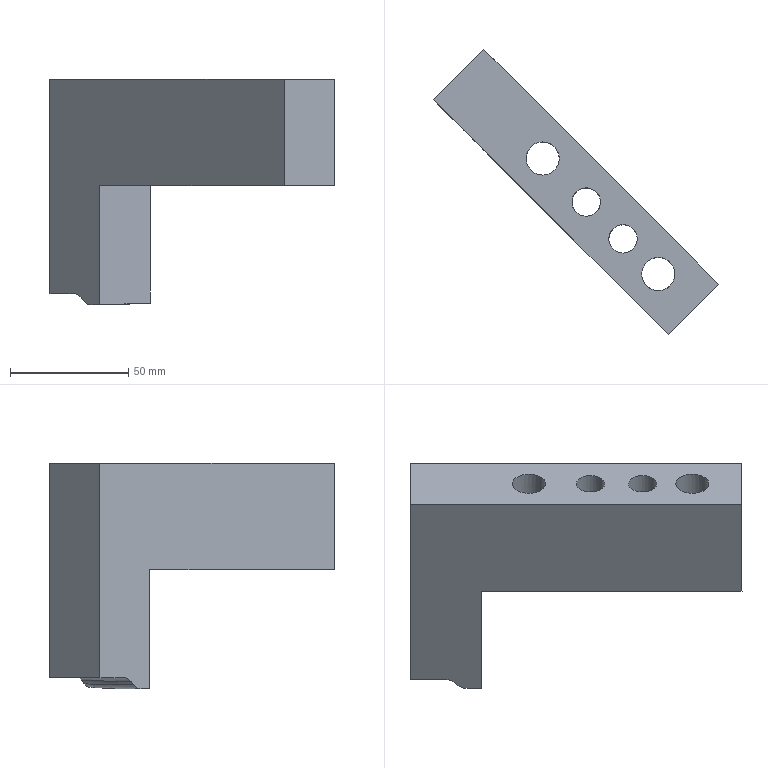Part | NX | features solid 2 | 1 solid | 21 faces | box 120.302 x 120.208 x 95.322 mm | volume 201033 mm3 | spline 8 | plane 7 | cylinder 6 | commonest cylinder face diameters 12 x2 14 x2 20 x2
STEP:
#1=CARTESIAN_POINT('',(-245.691,302.804,55.));
#2=VERTEX_POINT('',#1);
#3=CARTESIAN_POINT('',(-249.934,307.047,55.));
#4=DIRECTION('',(0.,0.,1.));
#5=DIRECTION('',(0.7071,-0.7071,0.));
#6=AXIS2_PLACEMENT_3D('',#3,#4,#5);
#7=CIRCLE('',#6,6.);
#8=EDGE_CURVE('',#2,#2,#7,.T.);
#9=ORIENTED_EDGE('',*,*,#8,.T.);
#10=EDGE_LOOP('',(#9));
#11=FACE_BOUND('',#10,.T.);
#12=CARTESIAN_POINT('',(-276.804,333.917,55.));
#13=VERTEX_POINT('',#12);
#14=CARTESIAN_POINT('',(-283.875,340.988,55.));
#15=DIRECTION('',(0.,0.,1.));
#16=DIRECTION('',(0.7071,-0.7071,0.));
#17=AXIS2_PLACEMENT_3D('',#14,#15,#16);
#18=CIRCLE('',#17,10.);
#19=EDGE_CURVE('',#13,#13,#18,.T.);
#20=ORIENTED_EDGE('',*,*,#19,.T.);
#21=EDGE_LOOP('',(#20));
#22=FACE_BOUND('',#21,.T.);
#23=CARTESIAN_POINT('',(-228.013,285.126,55.));
#24=VERTEX_POINT('',#23);
#25=CARTESIAN_POINT('',(-235.084,292.198,55.));
#26=DIRECTION('',(0.,0.,1.));
#27=DIRECTION('',(0.7071,-0.7071,0.));
#28=AXIS2_PLACEMENT_3D('',#25,#26,#27);
#29=CIRCLE('',#28,10.);
#30=EDGE_CURVE('',#24,#24,#29,.T.);
#31=ORIENTED_EDGE('',*,*,#30,.T.);
#32=EDGE_LOOP('',(#31));
#33=FACE_BOUND('',#32,.T.);
#34=CARTESIAN_POINT('',(-261.247,318.36,55.));
#35=VERTEX_POINT('',#34);
#36=CARTESIAN_POINT('',(-265.49,322.603,55.));
#37=DIRECTION('',(0.,0.,1.));
#38=DIRECTION('',(0.7071,-0.7071,0.));
#39=AXIS2_PLACEMENT_3D('',#36,#37,#38);
#40=CIRCLE('',#39,6.);
#41=EDGE_CURVE('',#35,#35,#40,.T.);
#42=ORIENTED_EDGE('',*,*,#41,.T.);
#43=EDGE_LOOP('',(#42));
#44=FACE_BOUND('',#43,.T.);
#45=CARTESIAN_POINT('',(-230.875,266.775,55.));
#46=VERTEX_POINT('',#45);
#47=CARTESIAN_POINT('',(-308.751,344.651,55.));
#48=VERTEX_POINT('',#47);
#49=CARTESIAN_POINT('',(-244.984,280.884,55.));
#50=DIRECTION('',(0.7071,-0.7071,0.));
#51=VECTOR('',#50,1000.);
#52=LINE('',#49,#51);
#53=EDGE_CURVE('',#46,#48,#52,.F.);
#54=ORIENTED_EDGE('',*,*,#53,.T.);
#55=CARTESIAN_POINT('',(-287.444,365.77,55.));
#56=VERTEX_POINT('',#55);
#57=CARTESIAN_POINT('',(-308.751,344.651,55.));
#58=CARTESIAN_POINT('',(-301.65,351.692,55.));
#59=CARTESIAN_POINT('',(-294.548,358.732,55.));
#60=CARTESIAN_POINT('',(-287.444,365.77,55.));
#61=B_SPLINE_CURVE_WITH_KNOTS('',3,(#57,#58,#59,#60),.UNSPECIFIED.,.F.,.F.,(4,4),(0.,0.03),.UNSPECIFIED.);
#62=EDGE_CURVE('',#48,#56,#61,.T.);
#63=ORIENTED_EDGE('',*,*,#62,.T.);
#64=CARTESIAN_POINT('',(-209.662,287.989,55.));
#65=VERTEX_POINT('',#64);
#66=CARTESIAN_POINT('',(-223.771,302.097,55.));
#67=DIRECTION('',(0.7071,-0.7071,0.));
#68=VECTOR('',#67,1000.);
#69=LINE('',#66,#68);
#70=EDGE_CURVE('',#65,#56,#69,.F.);
#71=ORIENTED_EDGE('',*,*,#70,.F.);
#72=CARTESIAN_POINT('',(-259.16,238.491,55.));
#73=DIRECTION('',(-0.7071,-0.7071,0.));
#74=VECTOR('',#73,1000.);
#75=LINE('',#72,#74);
#76=EDGE_CURVE('',#46,#65,#75,.F.);
#77=ORIENTED_EDGE('',*,*,#76,.F.);
#78=EDGE_LOOP('',(#54,#63,#71,#77));
#79=FACE_BOUND('',#78,.T.);
#80=CARTESIAN_POINT('',(-244.984,280.884,55.));
#81=DIRECTION('',(0.,0.,1.));
#82=DIRECTION('',(0.7071,0.7071,0.));
#83=AXIS2_PLACEMENT_3D('',#80,#81,#82);
#84=PLANE('',#83);
#85=ADVANCED_FACE('',(#11,#22,#33,#44,#79),#84,.F.);
#86=CARTESIAN_POINT('',(-329.964,365.864,100.));
#87=VERTEX_POINT('',#86);
#88=CARTESIAN_POINT('',(-308.657,386.983,100.));
#89=VERTEX_POINT('',#88);
#90=CARTESIAN_POINT('',(-329.964,365.864,100.));
#91=CARTESIAN_POINT('',(-322.863,372.905,100.));
#92=CARTESIAN_POINT('',(-315.761,379.945,100.));
#93=CARTESIAN_POINT('',(-308.657,386.983,100.));
#94=B_SPLINE_CURVE_WITH_KNOTS('',3,(#90,#91,#92,#93),.UNSPECIFIED.,.F.,.F.,(4,4),(0.04583,0.07583),.UNSPECIFIED.);
#95=EDGE_CURVE('',#87,#89,#94,.T.);
#96=ORIENTED_EDGE('',*,*,#95,.F.);
#97=CARTESIAN_POINT('',(-230.875,266.775,100.));
#98=VERTEX_POINT('',#97);
#99=CARTESIAN_POINT('',(-322.766,358.666,100.));
#100=DIRECTION('',(-0.7071,0.7071,0.));
#101=VECTOR('',#100,1000.);
#102=LINE('',#99,#101);
#103=EDGE_CURVE('',#98,#87,#102,.T.);
#104=ORIENTED_EDGE('',*,*,#103,.F.);
#105=CARTESIAN_POINT('',(-209.662,287.989,100.));
#106=VERTEX_POINT('',#105);
#107=CARTESIAN_POINT('',(-177.842,319.808,100.));
#108=DIRECTION('',(0.7071,0.7071,0.));
#109=VECTOR('',#108,1000.);
#110=LINE('',#107,#109);
#111=EDGE_CURVE('',#98,#106,#110,.T.);
#112=ORIENTED_EDGE('',*,*,#111,.T.);
#113=CARTESIAN_POINT('',(-301.552,379.879,100.));
#114=DIRECTION('',(-0.7071,0.7071,0.));
#115=VECTOR('',#114,1000.);
#116=LINE('',#113,#115);
#117=EDGE_CURVE('',#106,#89,#116,.T.);
#118=ORIENTED_EDGE('',*,*,#117,.T.);
#119=EDGE_LOOP('',(#96,#104,#112,#118));
#120=FACE_BOUND('',#119,.T.);
#121=CARTESIAN_POINT('',(-249.934,301.047,100.));
#122=VERTEX_POINT('',#121);
#123=CARTESIAN_POINT('',(-249.934,307.047,100.));
#124=DIRECTION('',(0.,0.,1.));
#125=DIRECTION('',(0.,-1.,0.));
#126=AXIS2_PLACEMENT_3D('',#123,#124,#125);
#127=CIRCLE('',#126,6.);
#128=EDGE_CURVE('',#122,#122,#127,.T.);
#129=ORIENTED_EDGE('',*,*,#128,.F.);
#130=EDGE_LOOP('',(#129));
#131=FACE_BOUND('',#130,.T.);
#132=CARTESIAN_POINT('',(-235.084,285.198,100.));
#133=VERTEX_POINT('',#132);
#134=CARTESIAN_POINT('',(-235.084,292.198,100.));
#135=DIRECTION('',(0.,0.,1.));
#136=DIRECTION('',(0.,-1.,0.));
#137=AXIS2_PLACEMENT_3D('',#134,#135,#136);
#138=CIRCLE('',#137,7.);
#139=EDGE_CURVE('',#133,#133,#138,.T.);
#140=ORIENTED_EDGE('',*,*,#139,.F.);
#141=EDGE_LOOP('',(#140));
#142=FACE_BOUND('',#141,.T.);
#143=CARTESIAN_POINT('',(-283.875,333.988,100.));
#144=VERTEX_POINT('',#143);
#145=CARTESIAN_POINT('',(-283.875,340.988,100.));
#146=DIRECTION('',(0.,0.,1.));
#147=DIRECTION('',(0.,-1.,0.));
#148=AXIS2_PLACEMENT_3D('',#145,#146,#147);
#149=CIRCLE('',#148,7.);
#150=EDGE_CURVE('',#144,#144,#149,.T.);
#151=ORIENTED_EDGE('',*,*,#150,.F.);
#152=EDGE_LOOP('',(#151));
#153=FACE_BOUND('',#152,.T.);
#154=CARTESIAN_POINT('',(-265.49,316.603,100.));
#155=VERTEX_POINT('',#154);
#156=CARTESIAN_POINT('',(-265.49,322.603,100.));
#157=DIRECTION('',(0.,0.,1.));
#158=DIRECTION('',(0.,-1.,0.));
#159=AXIS2_PLACEMENT_3D('',#156,#157,#158);
#160=CIRCLE('',#159,6.);
#161=EDGE_CURVE('',#155,#155,#160,.T.);
#162=ORIENTED_EDGE('',*,*,#161,.F.);
#163=EDGE_LOOP('',(#162));
#164=FACE_BOUND('',#163,.T.);
#165=CARTESIAN_POINT('',(-269.733,411.699,100.));
#166=DIRECTION('',(0.,0.,1.));
#167=DIRECTION('',(0.7071,-0.7071,0.));
#168=AXIS2_PLACEMENT_3D('',#165,#166,#167);
#169=PLANE('',#168);
#170=ADVANCED_FACE('',(#120,#131,#142,#153,#164),#169,.T.);
#171=CARTESIAN_POINT('',(-230.875,266.775,75.));
#172=DIRECTION('',(0.,0.,1.));
#173=VECTOR('',#172,1000.);
#174=LINE('',#171,#173);
#175=EDGE_CURVE('',#46,#98,#174,.T.);
#176=ORIENTED_EDGE('',*,*,#175,.F.);
#177=ORIENTED_EDGE('',*,*,#76,.T.);
#178=CARTESIAN_POINT('',(-209.662,287.989,75.));
#179=DIRECTION('',(0.,0.,1.));
#180=VECTOR('',#179,1000.);
#181=LINE('',#178,#180);
#182=EDGE_CURVE('',#65,#106,#181,.T.);
#183=ORIENTED_EDGE('',*,*,#182,.T.);
#184=ORIENTED_EDGE('',*,*,#111,.F.);
#185=EDGE_LOOP('',(#176,#177,#183,#184));
#186=FACE_BOUND('',#185,.T.);
#187=CARTESIAN_POINT('',(-259.16,238.491,75.));
#188=DIRECTION('',(0.7071,-0.7071,0.));
#189=DIRECTION('',(0.,0.,-1.));
#190=AXIS2_PLACEMENT_3D('',#187,#188,#189);
#191=PLANE('',#190);
#192=ADVANCED_FACE('',(#186),#191,.T.);
#193=CARTESIAN_POINT('',(-312.943,348.843,4.801));
#194=VERTEX_POINT('',#193);
#195=CARTESIAN_POINT('',(-315.708,351.608,6.413));
#196=VERTEX_POINT('',#195);
#197=CARTESIAN_POINT('',(-312.942,348.842,4.801));
#198=CARTESIAN_POINT('',(-313.969,349.869,4.845));
#199=CARTESIAN_POINT('',(-314.962,350.862,5.425));
#200=CARTESIAN_POINT('',(-315.711,351.611,6.417));
#201=B_SPLINE_CURVE_WITH_KNOTS('',3,(#197,#198,#199,#200),.UNSPECIFIED.,.F.,.F.,(4,4),(0.,0.004334),.UNSPECIFIED.);
#202=EDGE_CURVE('',#194,#196,#201,.T.);
#203=ORIENTED_EDGE('',*,*,#202,.F.);
#204=CARTESIAN_POINT('',(-308.751,344.651,4.678));
#205=VERTEX_POINT('',#204);
#206=CARTESIAN_POINT('',(-312.944,348.844,4.801));
#207=CARTESIAN_POINT('',(-311.546,347.446,4.74));
#208=CARTESIAN_POINT('',(-310.149,346.049,4.7));
#209=CARTESIAN_POINT('',(-308.751,344.651,4.678));
#210=B_SPLINE_CURVE_WITH_KNOTS('',3,(#206,#207,#208,#209),.UNSPECIFIED.,.F.,.F.,(4,4),(0.02411,0.03004),.UNSPECIFIED.);
#211=EDGE_CURVE('',#194,#205,#210,.T.);
#212=ORIENTED_EDGE('',*,*,#211,.T.);
#213=CARTESIAN_POINT('',(-308.751,344.651,54.885));
#214=DIRECTION('',(0.,0.,-1.));
#215=VECTOR('',#214,1000.);
#216=LINE('',#213,#215);
#217=EDGE_CURVE('',#48,#205,#216,.T.);
#218=ORIENTED_EDGE('',*,*,#217,.F.);
#219=ORIENTED_EDGE('',*,*,#53,.F.);
#220=ORIENTED_EDGE('',*,*,#175,.T.);
#221=ORIENTED_EDGE('',*,*,#103,.T.);
#222=CARTESIAN_POINT('',(-329.964,365.864,9.341));
#223=VERTEX_POINT('',#222);
#224=CARTESIAN_POINT('',(-329.964,365.864,70.));
#225=DIRECTION('',(0.,0.,-1.));
#226=VECTOR('',#225,1000.);
#227=LINE('',#224,#226);
#228=EDGE_CURVE('',#87,#223,#227,.T.);
#229=ORIENTED_EDGE('',*,*,#228,.T.);
#230=CARTESIAN_POINT('',(-328.671,364.571,9.579));
#231=VERTEX_POINT('',#230);
#232=CARTESIAN_POINT('',(-329.964,365.864,9.341));
#233=CARTESIAN_POINT('',(-329.542,365.442,9.515));
#234=CARTESIAN_POINT('',(-329.111,365.011,9.594));
#235=CARTESIAN_POINT('',(-328.672,364.572,9.579));
#236=B_SPLINE_CURVE_WITH_KNOTS('',3,(#232,#233,#234,#235),.UNSPECIFIED.,.F.,.F.,(4,4),(0.,0.001844),.UNSPECIFIED.);
#237=EDGE_CURVE('',#223,#231,#236,.T.);
#238=ORIENTED_EDGE('',*,*,#237,.T.);
#239=CARTESIAN_POINT('',(-319.575,355.475,9.376));
#240=VERTEX_POINT('',#239);
#241=CARTESIAN_POINT('',(-328.669,364.569,9.579));
#242=CARTESIAN_POINT('',(-325.638,361.538,9.472));
#243=CARTESIAN_POINT('',(-322.607,358.507,9.405));
#244=CARTESIAN_POINT('',(-319.575,355.475,9.376));
#245=B_SPLINE_CURVE_WITH_KNOTS('',3,(#241,#242,#243,#244),.UNSPECIFIED.,.F.,.F.,(4,4),(0.001832,0.01469),.UNSPECIFIED.);
#246=EDGE_CURVE('',#231,#240,#245,.T.);
#247=ORIENTED_EDGE('',*,*,#246,.T.);
#248=CARTESIAN_POINT('',(-316.651,352.551,7.683));
#249=VERTEX_POINT('',#248);
#250=CARTESIAN_POINT('',(-319.576,355.476,9.376));
#251=CARTESIAN_POINT('',(-318.489,354.389,9.366));
#252=CARTESIAN_POINT('',(-317.43,353.33,8.753));
#253=CARTESIAN_POINT('',(-316.65,352.55,7.682));
#254=B_SPLINE_CURVE_WITH_KNOTS('',3,(#250,#251,#252,#253),.UNSPECIFIED.,.F.,.F.,(4,4),(0.,0.004586),.UNSPECIFIED.);
#255=EDGE_CURVE('',#240,#249,#254,.T.);
#256=ORIENTED_EDGE('',*,*,#255,.T.);
#257=CARTESIAN_POINT('',(-316.651,352.551,7.683));
#258=CARTESIAN_POINT('',(-316.339,352.239,7.255));
#259=CARTESIAN_POINT('',(-316.024,351.924,6.831));
#260=CARTESIAN_POINT('',(-315.707,351.607,6.411));
#261=B_SPLINE_CURVE_WITH_KNOTS('',3,(#257,#258,#259,#260),.UNSPECIFIED.,.F.,.F.,(4,4),(0.01484,0.01668),.UNSPECIFIED.);
#262=EDGE_CURVE('',#249,#196,#261,.T.);
#263=ORIENTED_EDGE('',*,*,#262,.T.);
#264=EDGE_LOOP('',(#203,#212,#218,#219,#220,#221,#229,#238,#247,#256,#263));
#265=FACE_BOUND('',#264,.T.);
#266=CARTESIAN_POINT('',(-266.197,302.097,75.));
#267=DIRECTION('',(0.7071,0.7071,0.));
#268=DIRECTION('',(0.,0.,1.));
#269=AXIS2_PLACEMENT_3D('',#266,#267,#268);
#270=PLANE('',#269);
#271=ADVANCED_FACE('',(#265),#270,.F.);
#272=CARTESIAN_POINT('',(-291.158,369.484,5.289));
#273=VERTEX_POINT('',#272);
#274=CARTESIAN_POINT('',(-287.444,365.77,5.473));
#275=VERTEX_POINT('',#274);
#276=CARTESIAN_POINT('',(-291.157,369.484,5.289));
#277=CARTESIAN_POINT('',(-289.919,368.246,5.342));
#278=CARTESIAN_POINT('',(-288.681,367.008,5.403));
#279=CARTESIAN_POINT('',(-287.444,365.77,5.473));
#280=B_SPLINE_CURVE_WITH_KNOTS('',3,(#276,#277,#278,#279),.UNSPECIFIED.,.F.,.F.,(4,4),(0.01502,0.02027),.UNSPECIFIED.);
#281=EDGE_CURVE('',#273,#275,#280,.T.);
#282=ORIENTED_EDGE('',*,*,#281,.F.);
#283=CARTESIAN_POINT('',(-294.149,372.475,6.862));
#284=VERTEX_POINT('',#283);
#285=CARTESIAN_POINT('',(-291.158,369.484,5.289));
#286=CARTESIAN_POINT('',(-292.256,370.582,5.242));
#287=CARTESIAN_POINT('',(-293.342,371.668,5.814));
#288=CARTESIAN_POINT('',(-294.151,372.477,6.865));
#289=B_SPLINE_CURVE_WITH_KNOTS('',3,(#285,#286,#287,#288),.UNSPECIFIED.,.F.,.F.,(4,4),(0.,0.004637),.UNSPECIFIED.);
#290=EDGE_CURVE('',#273,#284,#289,.T.);
#291=ORIENTED_EDGE('',*,*,#290,.T.);
#292=CARTESIAN_POINT('',(-295.242,373.569,8.306));
#293=VERTEX_POINT('',#292);
#294=CARTESIAN_POINT('',(-295.242,373.569,8.306));
#295=CARTESIAN_POINT('',(-294.88,373.206,7.819));
#296=CARTESIAN_POINT('',(-294.515,372.841,7.337));
#297=CARTESIAN_POINT('',(-294.146,372.473,6.858));
#298=B_SPLINE_CURVE_WITH_KNOTS('',3,(#294,#295,#296,#297),.UNSPECIFIED.,.F.,.F.,(4,4),(0.008363,0.01048),.UNSPECIFIED.);
#299=EDGE_CURVE('',#293,#284,#298,.T.);
#300=ORIENTED_EDGE('',*,*,#299,.F.);
#301=CARTESIAN_POINT('',(-298.297,376.624,9.952));
#302=VERTEX_POINT('',#301);
#303=CARTESIAN_POINT('',(-298.297,376.624,9.952));
#304=CARTESIAN_POINT('',(-297.172,375.498,10.002));
#305=CARTESIAN_POINT('',(-296.058,374.385,9.403));
#306=CARTESIAN_POINT('',(-295.242,373.568,8.306));
#307=B_SPLINE_CURVE_WITH_KNOTS('',3,(#303,#304,#305,#306),.UNSPECIFIED.,.F.,.F.,(4,4),(0.,0.004753),.UNSPECIFIED.);
#308=EDGE_CURVE('',#302,#293,#307,.T.);
#309=ORIENTED_EDGE('',*,*,#308,.F.);
#310=CARTESIAN_POINT('',(-307.448,385.775,9.639));
#311=VERTEX_POINT('',#310);
#312=CARTESIAN_POINT('',(-307.448,385.775,9.639));
#313=CARTESIAN_POINT('',(-304.397,382.724,9.71));
#314=CARTESIAN_POINT('',(-301.347,379.674,9.815));
#315=CARTESIAN_POINT('',(-298.298,376.624,9.952));
#316=B_SPLINE_CURVE_WITH_KNOTS('',3,(#312,#313,#314,#315),.UNSPECIFIED.,.F.,.F.,(4,4),(0.001709,0.01465),.UNSPECIFIED.);
#317=EDGE_CURVE('',#311,#302,#316,.T.);
#318=ORIENTED_EDGE('',*,*,#317,.F.);
#319=CARTESIAN_POINT('',(-308.657,386.983,9.361));
#320=VERTEX_POINT('',#319);
#321=CARTESIAN_POINT('',(-308.657,386.983,9.361));
#322=CARTESIAN_POINT('',(-308.264,386.59,9.537));
#323=CARTESIAN_POINT('',(-307.861,386.187,9.63));
#324=CARTESIAN_POINT('',(-307.448,385.775,9.639));
#325=B_SPLINE_CURVE_WITH_KNOTS('',3,(#321,#322,#323,#324),.UNSPECIFIED.,.F.,.F.,(4,4),(0.,0.001732),.UNSPECIFIED.);
#326=EDGE_CURVE('',#320,#311,#325,.T.);
#327=ORIENTED_EDGE('',*,*,#326,.F.);
#328=CARTESIAN_POINT('',(-308.657,386.983,500.));
#329=DIRECTION('',(0.,0.,-1.));
#330=VECTOR('',#329,1000.);
#331=LINE('',#328,#330);
#332=EDGE_CURVE('',#89,#320,#331,.T.);
#333=ORIENTED_EDGE('',*,*,#332,.F.);
#334=ORIENTED_EDGE('',*,*,#117,.F.);
#335=ORIENTED_EDGE('',*,*,#182,.F.);
#336=ORIENTED_EDGE('',*,*,#70,.T.);
#337=CARTESIAN_POINT('',(-287.444,365.77,55.532));
#338=DIRECTION('',(0.,0.,-1.));
#339=VECTOR('',#338,1000.);
#340=LINE('',#337,#339);
#341=EDGE_CURVE('',#56,#275,#340,.T.);
#342=ORIENTED_EDGE('',*,*,#341,.T.);
#343=EDGE_LOOP('',(#282,#291,#300,#309,#318,#327,#333,#334,#335,#336,#342));
#344=FACE_BOUND('',#343,.T.);
#345=CARTESIAN_POINT('',(-244.984,323.31,-200.));
#346=DIRECTION('',(0.7071,0.7071,0.));
#347=DIRECTION('',(0.,0.,1.));
#348=AXIS2_PLACEMENT_3D('',#345,#346,#347);
#349=PLANE('',#348);
#350=ADVANCED_FACE('',(#344),#349,.T.);
#351=CARTESIAN_POINT('',(-228.013,285.126,75.));
#352=VERTEX_POINT('',#351);
#353=CARTESIAN_POINT('',(-235.084,292.198,75.));
#354=DIRECTION('',(0.,0.,1.));
#355=DIRECTION('',(0.7071,-0.7071,0.));
#356=AXIS2_PLACEMENT_3D('',#353,#354,#355);
#357=CIRCLE('',#356,10.);
#358=EDGE_CURVE('',#352,#352,#357,.F.);
#359=ORIENTED_EDGE('',*,*,#358,.F.);
#360=EDGE_LOOP('',(#359));
#361=FACE_BOUND('',#360,.T.);
#362=ORIENTED_EDGE('',*,*,#30,.F.);
#363=EDGE_LOOP('',(#362));
#364=FACE_BOUND('',#363,.T.);
#365=CARTESIAN_POINT('',(-235.084,292.198,72.));
#366=DIRECTION('',(0.,0.,-1.));
#367=DIRECTION('',(0.7071,-0.7071,0.));
#368=AXIS2_PLACEMENT_3D('',#365,#366,#367);
#369=CYLINDRICAL_SURFACE('',#368,10.);
#370=ADVANCED_FACE('',(#361,#364),#369,.F.);
#371=CARTESIAN_POINT('',(-276.804,333.917,75.));
#372=VERTEX_POINT('',#371);
#373=CARTESIAN_POINT('',(-283.875,340.988,75.));
#374=DIRECTION('',(0.,0.,-1.));
#375=DIRECTION('',(0.7071,-0.7071,0.));
#376=AXIS2_PLACEMENT_3D('',#373,#374,#375);
#377=CIRCLE('',#376,10.);
#378=EDGE_CURVE('',#372,#372,#377,.T.);
#379=ORIENTED_EDGE('',*,*,#378,.F.);
#380=EDGE_LOOP('',(#379));
#381=FACE_BOUND('',#380,.T.);
#382=ORIENTED_EDGE('',*,*,#19,.F.);
#383=EDGE_LOOP('',(#382));
#384=FACE_BOUND('',#383,.T.);
#385=CARTESIAN_POINT('',(-283.875,340.988,75.));
#386=DIRECTION('',(0.,0.,-1.));
#387=DIRECTION('',(0.7071,-0.7071,0.));
#388=AXIS2_PLACEMENT_3D('',#385,#386,#387);
#389=CYLINDRICAL_SURFACE('',#388,10.);
#390=ADVANCED_FACE('',(#381,#384),#389,.F.);
#391=ORIENTED_EDGE('',*,*,#332,.T.);
#392=CARTESIAN_POINT('',(-308.657,386.983,9.361));
#393=CARTESIAN_POINT('',(-315.76,379.946,9.178));
#394=CARTESIAN_POINT('',(-322.864,372.905,9.162));
#395=CARTESIAN_POINT('',(-329.964,365.864,9.341));
#396=B_SPLINE_CURVE_WITH_KNOTS('',3,(#392,#393,#394,#395),.UNSPECIFIED.,.F.,.F.,(4,4),(0.,0.03),.UNSPECIFIED.);
#397=EDGE_CURVE('',#320,#223,#396,.T.);
#398=ORIENTED_EDGE('',*,*,#397,.T.);
#399=ORIENTED_EDGE('',*,*,#228,.F.);
#400=ORIENTED_EDGE('',*,*,#95,.T.);
#401=EDGE_LOOP('',(#391,#398,#399,#400));
#402=FACE_BOUND('',#401,.T.);
#403=CARTESIAN_POINT('',(-308.657,386.983,100.));
#404=CARTESIAN_POINT('',(-308.657,386.983,8.651));
#405=CARTESIAN_POINT('',(-315.763,379.943,100.));
#406=CARTESIAN_POINT('',(-315.763,379.943,8.651));
#407=CARTESIAN_POINT('',(-322.865,372.903,100.));
#408=CARTESIAN_POINT('',(-322.865,372.903,8.651));
#409=CARTESIAN_POINT('',(-329.964,365.864,100.));
#410=CARTESIAN_POINT('',(-329.964,365.864,8.651));
#411=B_SPLINE_SURFACE_WITH_KNOTS('',3,1,((#403,#404),(#405,#406),(#407,#408),(#409,#410)),.SURF_OF_LINEAR_EXTRUSION.,.F.,.F.,.F.,(4,4),(2,2),(0.9474,0.9616),(0.,1.),.PIECEWISE_BEZIER_KNOTS.);
#412=ADVANCED_FACE('',(#402),#411,.F.);
#413=CARTESIAN_POINT('',(-230.135,287.248,75.));
#414=VERTEX_POINT('',#413);
#415=CARTESIAN_POINT('',(-235.084,292.198,75.));
#416=DIRECTION('',(0.,0.,1.));
#417=DIRECTION('',(0.7071,-0.7071,0.));
#418=AXIS2_PLACEMENT_3D('',#415,#416,#417);
#419=CIRCLE('',#418,7.);
#420=EDGE_CURVE('',#414,#414,#419,.T.);
#421=ORIENTED_EDGE('',*,*,#420,.T.);
#422=EDGE_LOOP('',(#421));
#423=FACE_BOUND('',#422,.T.);
#424=ORIENTED_EDGE('',*,*,#358,.T.);
#425=EDGE_LOOP('',(#424));
#426=FACE_BOUND('',#425,.T.);
#427=CARTESIAN_POINT('',(-235.084,292.198,75.));
#428=DIRECTION('',(0.,0.,1.));
#429=DIRECTION('',(-0.7071,0.7071,0.));
#430=AXIS2_PLACEMENT_3D('',#427,#428,#429);
#431=PLANE('',#430);
#432=ADVANCED_FACE('',(#423,#426),#431,.F.);
#433=ORIENTED_EDGE('',*,*,#139,.T.);
#434=EDGE_LOOP('',(#433));
#435=FACE_BOUND('',#434,.T.);
#436=ORIENTED_EDGE('',*,*,#420,.F.);
#437=EDGE_LOOP('',(#436));
#438=FACE_BOUND('',#437,.T.);
#439=CARTESIAN_POINT('',(-235.084,292.198,72.));
#440=DIRECTION('',(0.,0.,1.));
#441=DIRECTION('',(-0.7071,0.7071,0.));
#442=AXIS2_PLACEMENT_3D('',#439,#440,#441);
#443=CYLINDRICAL_SURFACE('',#442,7.);
#444=ADVANCED_FACE('',(#435,#438),#443,.F.);
#445=CARTESIAN_POINT('',(-278.925,336.038,75.));
#446=VERTEX_POINT('',#445);
#447=CARTESIAN_POINT('',(-283.875,340.988,75.));
#448=DIRECTION('',(0.,0.,1.));
#449=DIRECTION('',(0.7071,-0.7071,0.));
#450=AXIS2_PLACEMENT_3D('',#447,#448,#449);
#451=CIRCLE('',#450,7.);
#452=EDGE_CURVE('',#446,#446,#451,.T.);
#453=ORIENTED_EDGE('',*,*,#452,.T.);
#454=EDGE_LOOP('',(#453));
#455=FACE_BOUND('',#454,.T.);
#456=ORIENTED_EDGE('',*,*,#378,.T.);
#457=EDGE_LOOP('',(#456));
#458=FACE_BOUND('',#457,.T.);
#459=CARTESIAN_POINT('',(-283.875,340.988,75.));
#460=DIRECTION('',(0.,0.,1.));
#461=DIRECTION('',(-0.7071,0.7071,0.));
#462=AXIS2_PLACEMENT_3D('',#459,#460,#461);
#463=PLANE('',#462);
#464=ADVANCED_FACE('',(#455,#458),#463,.F.);
#465=ORIENTED_EDGE('',*,*,#150,.T.);
#466=EDGE_LOOP('',(#465));
#467=FACE_BOUND('',#466,.T.);
#468=ORIENTED_EDGE('',*,*,#452,.F.);
#469=EDGE_LOOP('',(#468));
#470=FACE_BOUND('',#469,.T.);
#471=CARTESIAN_POINT('',(-283.875,340.988,75.));
#472=DIRECTION('',(0.,0.,1.));
#473=DIRECTION('',(-0.7071,0.7071,0.));
#474=AXIS2_PLACEMENT_3D('',#471,#472,#473);
#475=CYLINDRICAL_SURFACE('',#474,7.);
#476=ADVANCED_FACE('',(#467,#470),#475,.F.);
#477=ORIENTED_EDGE('',*,*,#161,.T.);
#478=EDGE_LOOP('',(#477));
#479=FACE_BOUND('',#478,.T.);
#480=ORIENTED_EDGE('',*,*,#41,.F.);
#481=EDGE_LOOP('',(#480));
#482=FACE_BOUND('',#481,.T.);
#483=CARTESIAN_POINT('',(-265.49,322.603,105.));
#484=DIRECTION('',(0.,0.,-1.));
#485=DIRECTION('',(-0.7071,0.7071,0.));
#486=AXIS2_PLACEMENT_3D('',#483,#484,#485);
#487=CYLINDRICAL_SURFACE('',#486,6.);
#488=ADVANCED_FACE('',(#479,#482),#487,.F.);
#489=ORIENTED_EDGE('',*,*,#128,.T.);
#490=EDGE_LOOP('',(#489));
#491=FACE_BOUND('',#490,.T.);
#492=ORIENTED_EDGE('',*,*,#8,.F.);
#493=EDGE_LOOP('',(#492));
#494=FACE_BOUND('',#493,.T.);
#495=CARTESIAN_POINT('',(-249.934,307.047,105.));
#496=DIRECTION('',(0.,0.,-1.));
#497=DIRECTION('',(-0.7071,0.7071,0.));
#498=AXIS2_PLACEMENT_3D('',#495,#496,#497);
#499=CYLINDRICAL_SURFACE('',#498,6.);
#500=ADVANCED_FACE('',(#491,#494),#499,.F.);
#501=ORIENTED_EDGE('',*,*,#217,.T.);
#502=CARTESIAN_POINT('',(-308.751,344.651,4.678));
#503=CARTESIAN_POINT('',(-301.646,351.695,4.704));
#504=CARTESIAN_POINT('',(-294.541,358.738,4.937));
#505=CARTESIAN_POINT('',(-287.444,365.77,5.473));
#506=B_SPLINE_CURVE_WITH_KNOTS('',3,(#502,#503,#504,#505),.UNSPECIFIED.,.F.,.F.,(4,4),(0.,0.03001),.UNSPECIFIED.);
#507=EDGE_CURVE('',#205,#275,#506,.T.);
#508=ORIENTED_EDGE('',*,*,#507,.T.);
#509=ORIENTED_EDGE('',*,*,#341,.F.);
#510=ORIENTED_EDGE('',*,*,#62,.F.);
#511=EDGE_LOOP('',(#501,#508,#509,#510));
#512=FACE_BOUND('',#511,.T.);
#513=CARTESIAN_POINT('',(-308.751,344.651,55.));
#514=CARTESIAN_POINT('',(-308.751,344.651,4.377));
#515=CARTESIAN_POINT('',(-301.65,351.692,55.));
#516=CARTESIAN_POINT('',(-301.65,351.692,4.377));
#517=CARTESIAN_POINT('',(-294.55,358.729,55.));
#518=CARTESIAN_POINT('',(-294.55,358.729,4.377));
#519=CARTESIAN_POINT('',(-287.444,365.77,55.));
#520=CARTESIAN_POINT('',(-287.444,365.77,4.377));
#521=B_SPLINE_SURFACE_WITH_KNOTS('',3,1,((#513,#514),(#515,#516),(#517,#518),(#519,#520)),.SURF_OF_LINEAR_EXTRUSION.,.F.,.F.,.F.,(4,4),(2,2),(0.004227,1.005),(0.,1.),.PIECEWISE_BEZIER_KNOTS.);
#522=ADVANCED_FACE('',(#512),#521,.F.);
#523=ORIENTED_EDGE('',*,*,#202,.T.);
#524=CARTESIAN_POINT('',(-315.711,351.611,6.417));
#525=CARTESIAN_POINT('',(-312.154,355.059,6.353));
#526=CARTESIAN_POINT('',(-306.767,360.279,6.353));
#527=CARTESIAN_POINT('',(-299.594,367.218,6.57));
#528=CARTESIAN_POINT('',(-295.921,370.768,6.757));
#529=CARTESIAN_POINT('',(-294.151,372.477,6.865));
#530=B_SPLINE_CURVE_WITH_KNOTS('',3,(#524,#525,#526,#527,#528,#529),.UNSPECIFIED.,.F.,.F.,(4,1,1,4),(0.1993,0.2668,0.3006,0.3344),.UNSPECIFIED.);
#531=EDGE_CURVE('',#196,#284,#530,.T.);
#532=ORIENTED_EDGE('',*,*,#531,.T.);
#533=ORIENTED_EDGE('',*,*,#290,.F.);
#534=CARTESIAN_POINT('',(-291.158,369.484,5.289));
#535=CARTESIAN_POINT('',(-292.931,367.783,5.171));
#536=CARTESIAN_POINT('',(-296.636,364.246,4.966));
#537=CARTESIAN_POINT('',(-303.874,357.375,4.735));
#538=CARTESIAN_POINT('',(-309.334,352.229,4.736));
#539=CARTESIAN_POINT('',(-312.942,348.842,4.801));
#540=B_SPLINE_CURVE_WITH_KNOTS('',3,(#534,#535,#536,#537,#538,#539),.UNSPECIFIED.,.F.,.F.,(4,1,1,4),(0.6665,0.7002,0.7339,0.8013),.UNSPECIFIED.);
#541=EDGE_CURVE('',#194,#273,#540,.F.);
#542=ORIENTED_EDGE('',*,*,#541,.F.);
#543=EDGE_LOOP('',(#523,#532,#533,#542));
#544=FACE_BOUND('',#543,.T.);
#545=CARTESIAN_POINT('',(-291.015,369.621,5.298));
#546=CARTESIAN_POINT('',(-291.66,370.285,5.271));
#547=CARTESIAN_POINT('',(-292.315,370.947,5.422));
#548=CARTESIAN_POINT('',(-292.948,371.574,5.753));
#549=CARTESIAN_POINT('',(-293.526,372.132,6.247));
#550=CARTESIAN_POINT('',(-294.024,372.6,6.872));
#551=CARTESIAN_POINT('',(-291.411,369.241,5.272));
#552=CARTESIAN_POINT('',(-292.057,369.905,5.245));
#553=CARTESIAN_POINT('',(-292.711,370.566,5.397));
#554=CARTESIAN_POINT('',(-293.344,371.193,5.728));
#555=CARTESIAN_POINT('',(-293.921,371.752,6.223));
#556=CARTESIAN_POINT('',(-294.418,372.219,6.848));
#557=CARTESIAN_POINT('',(-291.812,368.856,5.246));
#558=CARTESIAN_POINT('',(-292.457,369.52,5.22));
#559=CARTESIAN_POINT('',(-293.112,370.181,5.372));
#560=CARTESIAN_POINT('',(-293.744,370.808,5.704));
#561=CARTESIAN_POINT('',(-294.32,371.367,6.199));
#562=CARTESIAN_POINT('',(-294.817,371.835,6.825));
#563=CARTESIAN_POINT('',(-292.218,368.468,5.22));
#564=CARTESIAN_POINT('',(-292.862,369.131,5.195));
#565=CARTESIAN_POINT('',(-293.517,369.793,5.348));
#566=CARTESIAN_POINT('',(-294.148,370.419,5.68));
#567=CARTESIAN_POINT('',(-294.723,370.978,6.175));
#568=CARTESIAN_POINT('',(-295.219,371.446,6.801));
#569=CARTESIAN_POINT('',(-293.048,367.673,5.169));
#570=CARTESIAN_POINT('',(-293.693,368.336,5.146));
#571=CARTESIAN_POINT('',(-294.345,368.997,5.3));
#572=CARTESIAN_POINT('',(-294.975,369.623,5.633));
#573=CARTESIAN_POINT('',(-295.548,370.182,6.129));
#574=CARTESIAN_POINT('',(-296.041,370.651,6.755));
#575=CARTESIAN_POINT('',(-293.88,366.878,5.123));
#576=CARTESIAN_POINT('',(-294.524,367.541,5.1));
#577=CARTESIAN_POINT('',(-295.175,368.201,5.256));
#578=CARTESIAN_POINT('',(-295.802,368.828,5.59));
#579=CARTESIAN_POINT('',(-296.374,369.387,6.086));
#580=CARTESIAN_POINT('',(-296.864,369.856,6.713));
#581=CARTESIAN_POINT('',(-294.299,366.478,5.1));
#582=CARTESIAN_POINT('',(-294.942,367.141,5.079));
#583=CARTESIAN_POINT('',(-295.592,367.801,5.235));
#584=CARTESIAN_POINT('',(-296.219,368.427,5.57));
#585=CARTESIAN_POINT('',(-296.789,368.986,6.066));
#586=CARTESIAN_POINT('',(-297.279,369.455,6.692));
#587=CARTESIAN_POINT('',(-295.659,365.181,5.029));
#588=CARTESIAN_POINT('',(-296.3,365.842,5.011));
#589=CARTESIAN_POINT('',(-296.948,366.502,5.169));
#590=CARTESIAN_POINT('',(-297.571,367.127,5.505));
#591=CARTESIAN_POINT('',(-298.138,367.686,6.001));
#592=CARTESIAN_POINT('',(-298.624,368.155,6.627));
#593=CARTESIAN_POINT('',(-297.014,363.89,4.969));
#594=CARTESIAN_POINT('',(-297.654,364.55,4.953));
#595=CARTESIAN_POINT('',(-298.299,365.207,5.113));
#596=CARTESIAN_POINT('',(-298.919,365.831,5.45));
#597=CARTESIAN_POINT('',(-299.482,366.39,5.947));
#598=CARTESIAN_POINT('',(-299.965,366.859,6.571));
#599=CARTESIAN_POINT('',(-297.952,362.998,4.931));
#600=CARTESIAN_POINT('',(-298.591,363.656,4.918));
#601=CARTESIAN_POINT('',(-299.234,364.312,5.08));
#602=CARTESIAN_POINT('',(-299.852,364.935,5.417));
#603=CARTESIAN_POINT('',(-300.412,365.493,5.913));
#604=CARTESIAN_POINT('',(-300.892,365.963,6.537));
#605=CARTESIAN_POINT('',(-299.594,361.439,4.874));
#606=CARTESIAN_POINT('',(-300.229,362.094,4.864));
#607=CARTESIAN_POINT('',(-300.869,362.748,5.028));
#608=CARTESIAN_POINT('',(-301.482,363.369,5.366));
#609=CARTESIAN_POINT('',(-302.038,363.925,5.861));
#610=CARTESIAN_POINT('',(-302.513,364.395,6.483));
#611=CARTESIAN_POINT('',(-301.235,359.883,4.83));
#612=CARTESIAN_POINT('',(-301.867,360.535,4.824));
#613=CARTESIAN_POINT('',(-302.503,361.186,4.99));
#614=CARTESIAN_POINT('',(-303.111,361.804,5.329));
#615=CARTESIAN_POINT('',(-303.661,362.359,5.823));
#616=CARTESIAN_POINT('',(-304.132,362.828,6.443));
#617=CARTESIAN_POINT('',(-301.938,359.216,4.814));
#618=CARTESIAN_POINT('',(-302.569,359.867,4.81));
#619=CARTESIAN_POINT('',(-303.203,360.516,4.977));
#620=CARTESIAN_POINT('',(-303.809,361.134,5.315));
#621=CARTESIAN_POINT('',(-304.357,361.688,5.809));
#622=CARTESIAN_POINT('',(-304.825,362.157,6.427));
#623=CARTESIAN_POINT('',(-304.604,356.692,4.761));
#624=CARTESIAN_POINT('',(-305.23,357.337,4.764));
#625=CARTESIAN_POINT('',(-305.856,357.981,4.935));
#626=CARTESIAN_POINT('',(-306.453,358.593,5.274));
#627=CARTESIAN_POINT('',(-306.993,359.144,5.764));
#628=CARTESIAN_POINT('',(-307.454,359.612,6.378));
#629=CARTESIAN_POINT('',(-307.268,354.177,4.743));
#630=CARTESIAN_POINT('',(-307.887,354.816,4.753));
#631=CARTESIAN_POINT('',(-308.505,355.453,4.927));
#632=CARTESIAN_POINT('',(-309.093,356.059,5.266));
#633=CARTESIAN_POINT('',(-309.623,356.606,5.753));
#634=CARTESIAN_POINT('',(-310.076,357.072,6.36));
#635=CARTESIAN_POINT('',(-309.228,352.331,4.747));
#636=CARTESIAN_POINT('',(-309.841,352.965,4.762));
#637=CARTESIAN_POINT('',(-310.452,353.596,4.94));
#638=CARTESIAN_POINT('',(-311.033,354.198,5.278));
#639=CARTESIAN_POINT('',(-311.557,354.741,5.762));
#640=CARTESIAN_POINT('',(-312.003,355.205,6.364));
#641=CARTESIAN_POINT('',(-311.182,350.494,4.768));
#642=CARTESIAN_POINT('',(-311.79,351.121,4.789));
#643=CARTESIAN_POINT('',(-312.394,351.746,4.969));
#644=CARTESIAN_POINT('',(-312.968,352.342,5.307));
#645=CARTESIAN_POINT('',(-313.484,352.881,5.787));
#646=CARTESIAN_POINT('',(-313.925,353.343,6.384));
#647=CARTESIAN_POINT('',(-313.131,348.665,4.804));
#648=CARTESIAN_POINT('',(-313.733,349.286,4.831));
#649=CARTESIAN_POINT('',(-314.33,349.905,5.014));
#650=CARTESIAN_POINT('',(-314.896,350.494,5.351));
#651=CARTESIAN_POINT('',(-315.405,351.029,5.829));
#652=CARTESIAN_POINT('',(-315.839,351.487,6.419));
#653=B_SPLINE_SURFACE_WITH_KNOTS('',5,5,((#545,#546,#547,#548,#549,#550),(#551,#552,#553,#554,#555,#556),(#557,#558,#559,#560,#561,#562),(#563,#564,#565,#566,#567,#568),(#569,#570,#571,#572,#573,#574),(#575,#576,#577,#578,#579,#580),(#581,#582,#583,#584,#585,#586),(#587,#588,#589,#590,#591,#592),(#593,#594,#595,#596,#597,#598),(#599,#600,#601,#602,#603,#604),(#605,#606,#607,#608,#609,#610),(#611,#612,#613,#614,#615,#616),(#617,#618,#619,#620,#621,#622),(#623,#624,#625,#626,#627,#628),(#629,#630,#631,#632,#633,#634),(#635,#636,#637,#638,#639,#640),(#641,#642,#643,#644,#645,#646),(#647,#648,#649,#650,#651,#652)),.UNSPECIFIED.,.F.,.F.,.F.,(6,3,3,3,3,6),(6,6),(0.657,0.6694,0.6821,0.7107,0.7322,0.7921),(0.,1.),.UNSPECIFIED.);
#654=ADVANCED_FACE('',(#544),#653,.T.);
#655=CARTESIAN_POINT('',(-295.242,373.569,8.306));
#656=CARTESIAN_POINT('',(-297.213,371.661,8.191));
#657=CARTESIAN_POINT('',(-300.033,368.918,8.048));
#658=CARTESIAN_POINT('',(-303.564,365.467,7.908));
#659=CARTESIAN_POINT('',(-306.835,362.262,7.803));
#660=CARTESIAN_POINT('',(-311.124,358.041,7.71));
#661=CARTESIAN_POINT('',(-314.773,354.422,7.683));
#662=CARTESIAN_POINT('',(-316.651,352.551,7.683));
#663=B_SPLINE_CURVE_WITH_KNOTS('',3,(#655,#656,#657,#658,#659,#660,#661,#662),.UNSPECIFIED.,.F.,.F.,(4,1,1,1,1,4),(0.6944,0.727,0.7433,0.7597,0.7923,0.8249),.UNSPECIFIED.);
#664=EDGE_CURVE('',#293,#249,#663,.T.);
#665=ORIENTED_EDGE('',*,*,#664,.F.);
#666=ORIENTED_EDGE('',*,*,#299,.T.);
#667=ORIENTED_EDGE('',*,*,#531,.F.);
#668=ORIENTED_EDGE('',*,*,#262,.F.);
#669=EDGE_LOOP('',(#665,#666,#667,#668));
#670=FACE_BOUND('',#669,.T.);
#671=CARTESIAN_POINT('',(-294.772,373.94,8.274));
#672=CARTESIAN_POINT('',(-294.472,373.409,7.707));
#673=CARTESIAN_POINT('',(-294.169,372.873,7.145));
#674=CARTESIAN_POINT('',(-293.866,372.333,6.587));
#675=CARTESIAN_POINT('',(-293.266,371.266,5.504));
#676=CARTESIAN_POINT('',(-292.661,370.183,4.439));
#677=CARTESIAN_POINT('',(-292.363,369.647,3.921));
#678=CARTESIAN_POINT('',(-292.063,369.108,3.409));
#679=CARTESIAN_POINT('',(-291.761,368.565,2.901));
#680=CARTESIAN_POINT('',(-295.505,373.429,8.371));
#681=CARTESIAN_POINT('',(-295.205,372.899,7.803));
#682=CARTESIAN_POINT('',(-294.903,372.365,7.239));
#683=CARTESIAN_POINT('',(-294.599,371.826,6.68));
#684=CARTESIAN_POINT('',(-294.001,370.761,5.594));
#685=CARTESIAN_POINT('',(-293.396,369.68,4.527));
#686=CARTESIAN_POINT('',(-293.098,369.145,4.009));
#687=CARTESIAN_POINT('',(-292.799,368.607,3.495));
#688=CARTESIAN_POINT('',(-292.498,368.065,2.986));
#689=CARTESIAN_POINT('',(-296.237,372.917,8.47));
#690=CARTESIAN_POINT('',(-295.937,372.388,7.9));
#691=CARTESIAN_POINT('',(-295.635,371.855,7.335));
#692=CARTESIAN_POINT('',(-295.332,371.318,6.775));
#693=CARTESIAN_POINT('',(-294.735,370.255,5.686));
#694=CARTESIAN_POINT('',(-294.131,369.175,4.617));
#695=CARTESIAN_POINT('',(-293.833,368.642,4.097));
#696=CARTESIAN_POINT('',(-293.534,368.104,3.583));
#697=CARTESIAN_POINT('',(-293.233,367.563,3.073));
#698=CARTESIAN_POINT('',(-296.968,372.404,8.571));
#699=CARTESIAN_POINT('',(-296.668,371.876,8.));
#700=CARTESIAN_POINT('',(-296.367,371.344,7.433));
#701=CARTESIAN_POINT('',(-296.065,370.808,6.872));
#702=CARTESIAN_POINT('',(-295.468,369.747,5.78));
#703=CARTESIAN_POINT('',(-294.865,368.669,4.709));
#704=CARTESIAN_POINT('',(-294.567,368.137,4.188));
#705=CARTESIAN_POINT('',(-294.269,367.6,3.672));
#706=CARTESIAN_POINT('',(-293.968,367.059,3.161));
#707=CARTESIAN_POINT('',(-299.337,370.735,8.902));
#708=CARTESIAN_POINT('',(-299.039,370.211,8.326));
#709=CARTESIAN_POINT('',(-298.74,369.683,7.755));
#710=CARTESIAN_POINT('',(-298.438,369.15,7.19));
#711=CARTESIAN_POINT('',(-297.844,368.096,6.091));
#712=CARTESIAN_POINT('',(-297.243,367.024,5.012));
#713=CARTESIAN_POINT('',(-296.947,366.494,4.488));
#714=CARTESIAN_POINT('',(-296.649,365.961,3.969));
#715=CARTESIAN_POINT('',(-296.35,365.422,3.455));
#716=CARTESIAN_POINT('',(-301.702,369.054,9.248));
#717=CARTESIAN_POINT('',(-301.405,368.533,8.668));
#718=CARTESIAN_POINT('',(-301.107,368.008,8.094));
#719=CARTESIAN_POINT('',(-300.807,367.478,7.525));
#720=CARTESIAN_POINT('',(-300.215,366.43,6.418));
#721=CARTESIAN_POINT('',(-299.616,365.364,5.333));
#722=CARTESIAN_POINT('',(-299.321,364.837,4.805));
#723=CARTESIAN_POINT('',(-299.024,364.306,4.283));
#724=CARTESIAN_POINT('',(-298.725,363.77,3.766));
#725=CARTESIAN_POINT('',(-303.335,367.884,9.495));
#726=CARTESIAN_POINT('',(-303.039,367.366,8.913));
#727=CARTESIAN_POINT('',(-302.742,366.843,8.336));
#728=CARTESIAN_POINT('',(-302.442,366.315,7.764));
#729=CARTESIAN_POINT('',(-301.852,365.271,6.652));
#730=CARTESIAN_POINT('',(-301.254,364.209,5.562));
#731=CARTESIAN_POINT('',(-300.96,363.684,5.033));
#732=CARTESIAN_POINT('',(-300.663,363.154,4.509));
#733=CARTESIAN_POINT('',(-300.366,362.62,3.99));
#734=CARTESIAN_POINT('',(-307.465,364.907,10.14));
#735=CARTESIAN_POINT('',(-307.171,364.394,9.55));
#736=CARTESIAN_POINT('',(-306.876,363.877,8.966));
#737=CARTESIAN_POINT('',(-306.579,363.355,8.388));
#738=CARTESIAN_POINT('',(-305.992,362.321,7.265));
#739=CARTESIAN_POINT('',(-305.398,361.268,6.164));
#740=CARTESIAN_POINT('',(-305.105,360.747,5.629));
#741=CARTESIAN_POINT('',(-304.81,360.222,5.1));
#742=CARTESIAN_POINT('',(-304.514,359.692,4.576));
#743=CARTESIAN_POINT('',(-311.581,361.892,10.829));
#744=CARTESIAN_POINT('',(-311.289,361.385,10.233));
#745=CARTESIAN_POINT('',(-310.996,360.873,9.642));
#746=CARTESIAN_POINT('',(-310.701,360.356,9.058));
#747=CARTESIAN_POINT('',(-310.117,359.331,7.924));
#748=CARTESIAN_POINT('',(-309.527,358.288,6.812));
#749=CARTESIAN_POINT('',(-309.235,357.771,6.272));
#750=CARTESIAN_POINT('',(-308.942,357.25,5.738));
#751=CARTESIAN_POINT('',(-308.647,356.723,5.21));
#752=CARTESIAN_POINT('',(-314.067,360.054,11.261));
#753=CARTESIAN_POINT('',(-313.777,359.55,10.661));
#754=CARTESIAN_POINT('',(-313.484,359.042,10.067));
#755=CARTESIAN_POINT('',(-313.19,358.528,9.48));
#756=CARTESIAN_POINT('',(-312.609,357.509,8.338));
#757=CARTESIAN_POINT('',(-312.021,356.47,7.22));
#758=CARTESIAN_POINT('',(-311.73,355.956,6.678));
#759=CARTESIAN_POINT('',(-311.438,355.437,6.141));
#760=CARTESIAN_POINT('',(-311.144,354.914,5.61));
#761=CARTESIAN_POINT('',(-316.548,358.203,11.71));
#762=CARTESIAN_POINT('',(-316.259,357.703,11.106));
#763=CARTESIAN_POINT('',(-315.968,357.197,10.508));
#764=CARTESIAN_POINT('',(-315.675,356.686,9.917));
#765=CARTESIAN_POINT('',(-315.096,355.673,8.768));
#766=CARTESIAN_POINT('',(-314.51,354.64,7.643));
#767=CARTESIAN_POINT('',(-314.22,354.129,7.098));
#768=CARTESIAN_POINT('',(-313.929,353.613,6.558));
#769=CARTESIAN_POINT('',(-313.636,353.091,6.024));
#770=CARTESIAN_POINT('',(-319.023,356.336,12.177));
#771=CARTESIAN_POINT('',(-318.735,355.839,11.569));
#772=CARTESIAN_POINT('',(-318.446,355.337,10.967));
#773=CARTESIAN_POINT('',(-318.154,354.83,10.371));
#774=CARTESIAN_POINT('',(-317.578,353.824,9.214));
#775=CARTESIAN_POINT('',(-316.993,352.797,8.083));
#776=CARTESIAN_POINT('',(-316.705,352.288,7.534));
#777=CARTESIAN_POINT('',(-316.415,351.775,6.99));
#778=CARTESIAN_POINT('',(-316.123,351.256,6.453));
#779=B_SPLINE_SURFACE_WITH_KNOTS('',5,5,((#671,#672,#673,#674,#675,#676,#677,#678,#679),(#680,#681,#682,#683,#684,#685,#686,#687,#688),(#689,#690,#691,#692,#693,#694,#695,#696,#697),(#698,#699,#700,#701,#702,#703,#704,#705,#706),(#707,#708,#709,#710,#711,#712,#713,#714,#715),(#716,#717,#718,#719,#720,#721,#722,#723,#724),(#725,#726,#727,#728,#729,#730,#731,#732,#733),(#734,#735,#736,#737,#738,#739,#740,#741,#742),(#743,#744,#745,#746,#747,#748,#749,#750,#751),(#752,#753,#754,#755,#756,#757,#758,#759,#760),(#761,#762,#763,#764,#765,#766,#767,#768,#769),(#770,#771,#772,#773,#774,#775,#776,#777,#778)),.UNSPECIFIED.,.F.,.F.,.F.,(6,3,3,6),(6,3,6),(0.6924,0.7118,0.7554,0.8223),(0.3567,0.5394,0.7152),.UNSPECIFIED.);
#780=ADVANCED_FACE('',(#670),#779,.F.);
#781=CARTESIAN_POINT('',(-298.297,376.624,9.952));
#782=CARTESIAN_POINT('',(-305.442,369.666,9.574));
#783=CARTESIAN_POINT('',(-312.525,362.614,9.373));
#784=CARTESIAN_POINT('',(-319.576,355.476,9.376));
#785=B_SPLINE_CURVE_WITH_KNOTS('',3,(#781,#782,#783,#784),.UNSPECIFIED.,.F.,.F.,(4,4),(0.6951,0.8215),.UNSPECIFIED.);
#786=EDGE_CURVE('',#302,#240,#785,.T.);
#787=ORIENTED_EDGE('',*,*,#786,.F.);
#788=ORIENTED_EDGE('',*,*,#308,.T.);
#789=ORIENTED_EDGE('',*,*,#664,.T.);
#790=ORIENTED_EDGE('',*,*,#255,.F.);
#791=EDGE_LOOP('',(#787,#788,#789,#790));
#792=FACE_BOUND('',#791,.T.);
#793=CARTESIAN_POINT('',(-316.785,352.416,7.682));
#794=CARTESIAN_POINT('',(-317.249,352.882,8.32));
#795=CARTESIAN_POINT('',(-317.799,353.434,8.833));
#796=CARTESIAN_POINT('',(-318.412,354.05,9.188));
#797=CARTESIAN_POINT('',(-319.057,354.698,9.37));
#798=CARTESIAN_POINT('',(-319.703,355.347,9.376));
#799=CARTESIAN_POINT('',(-315.278,353.917,7.682));
#800=CARTESIAN_POINT('',(-315.744,354.384,8.322));
#801=CARTESIAN_POINT('',(-316.297,354.939,8.836));
#802=CARTESIAN_POINT('',(-316.913,355.557,9.191));
#803=CARTESIAN_POINT('',(-317.561,356.208,9.371));
#804=CARTESIAN_POINT('',(-318.209,356.861,9.375));
#805=CARTESIAN_POINT('',(-313.77,355.416,7.688));
#806=CARTESIAN_POINT('',(-314.239,355.884,8.331));
#807=CARTESIAN_POINT('',(-314.794,356.44,8.846));
#808=CARTESIAN_POINT('',(-315.413,357.061,9.202));
#809=CARTESIAN_POINT('',(-316.063,357.716,9.381));
#810=CARTESIAN_POINT('',(-316.713,358.371,9.382));
#811=CARTESIAN_POINT('',(-312.261,356.911,7.702));
#812=CARTESIAN_POINT('',(-312.732,357.38,8.347));
#813=CARTESIAN_POINT('',(-313.29,357.938,8.864));
#814=CARTESIAN_POINT('',(-313.912,358.562,9.22));
#815=CARTESIAN_POINT('',(-314.564,359.22,9.397));
#816=CARTESIAN_POINT('',(-315.216,359.878,9.396));
#817=CARTESIAN_POINT('',(-309.505,359.634,7.742));
#818=CARTESIAN_POINT('',(-309.981,360.104,8.391));
#819=CARTESIAN_POINT('',(-310.544,360.666,8.91));
#820=CARTESIAN_POINT('',(-311.171,361.295,9.267));
#821=CARTESIAN_POINT('',(-311.827,361.959,9.441));
#822=CARTESIAN_POINT('',(-312.482,362.623,9.435));
#823=CARTESIAN_POINT('',(-306.747,362.346,7.809));
#824=CARTESIAN_POINT('',(-307.227,362.819,8.461));
#825=CARTESIAN_POINT('',(-307.795,363.384,8.981));
#826=CARTESIAN_POINT('',(-308.425,364.018,9.337));
#827=CARTESIAN_POINT('',(-309.086,364.687,9.509));
#828=CARTESIAN_POINT('',(-309.742,365.356,9.498));
#829=CARTESIAN_POINT('',(-305.5,363.571,7.844));
#830=CARTESIAN_POINT('',(-305.982,364.044,8.497));
#831=CARTESIAN_POINT('',(-306.551,364.611,9.019));
#832=CARTESIAN_POINT('',(-307.184,365.246,9.374));
#833=CARTESIAN_POINT('',(-307.845,365.917,9.545));
#834=CARTESIAN_POINT('',(-308.502,366.589,9.532));
#835=CARTESIAN_POINT('',(-303.005,366.015,7.926));
#836=CARTESIAN_POINT('',(-303.491,366.49,8.581));
#837=CARTESIAN_POINT('',(-304.063,367.059,9.103));
#838=CARTESIAN_POINT('',(-304.699,367.699,9.458));
#839=CARTESIAN_POINT('',(-305.362,368.374,9.626));
#840=CARTESIAN_POINT('',(-306.02,369.05,9.608));
#841=CARTESIAN_POINT('',(-300.508,368.451,8.03));
#842=CARTESIAN_POINT('',(-300.997,368.928,8.686));
#843=CARTESIAN_POINT('',(-301.572,369.5,9.207));
#844=CARTESIAN_POINT('',(-302.21,370.143,9.56));
#845=CARTESIAN_POINT('',(-302.875,370.822,9.725));
#846=CARTESIAN_POINT('',(-303.533,371.501,9.704));
#847=CARTESIAN_POINT('',(-299.26,369.667,8.087));
#848=CARTESIAN_POINT('',(-299.749,370.144,8.743));
#849=CARTESIAN_POINT('',(-300.326,370.717,9.264));
#850=CARTESIAN_POINT('',(-300.965,371.362,9.616));
#851=CARTESIAN_POINT('',(-301.63,372.043,9.78));
#852=CARTESIAN_POINT('',(-302.288,372.725,9.757));
#853=CARTESIAN_POINT('',(-297.679,371.204,8.167));
#854=CARTESIAN_POINT('',(-298.17,371.681,8.822));
#855=CARTESIAN_POINT('',(-298.749,372.256,9.343));
#856=CARTESIAN_POINT('',(-299.389,372.902,9.693));
#857=CARTESIAN_POINT('',(-300.055,373.584,9.854));
#858=CARTESIAN_POINT('',(-300.712,374.267,9.829));
#859=CARTESIAN_POINT('',(-296.098,372.738,8.256));
#860=CARTESIAN_POINT('',(-296.592,373.216,8.91));
#861=CARTESIAN_POINT('',(-297.172,373.792,9.429));
#862=CARTESIAN_POINT('',(-297.812,374.439,9.777));
#863=CARTESIAN_POINT('',(-298.478,375.123,9.936));
#864=CARTESIAN_POINT('',(-299.135,375.807,9.908));
#865=CARTESIAN_POINT('',(-295.767,373.059,8.275));
#866=CARTESIAN_POINT('',(-296.261,373.538,8.929));
#867=CARTESIAN_POINT('',(-296.842,374.113,9.447));
#868=CARTESIAN_POINT('',(-297.482,374.761,9.795));
#869=CARTESIAN_POINT('',(-298.148,375.444,9.954));
#870=CARTESIAN_POINT('',(-298.805,376.129,9.925));
#871=CARTESIAN_POINT('',(-295.437,373.38,8.294));
#872=CARTESIAN_POINT('',(-295.931,373.859,8.948));
#873=CARTESIAN_POINT('',(-296.511,374.434,9.466));
#874=CARTESIAN_POINT('',(-297.152,375.082,9.813));
#875=CARTESIAN_POINT('',(-297.818,375.766,9.971));
#876=CARTESIAN_POINT('',(-298.474,376.451,9.942));
#877=CARTESIAN_POINT('',(-295.106,373.7,8.314));
#878=CARTESIAN_POINT('',(-295.601,374.179,8.967));
#879=CARTESIAN_POINT('',(-296.181,374.755,9.485));
#880=CARTESIAN_POINT('',(-296.822,375.403,9.832));
#881=CARTESIAN_POINT('',(-297.487,376.088,9.99));
#882=CARTESIAN_POINT('',(-298.143,376.773,9.96));
#883=B_SPLINE_SURFACE_WITH_KNOTS('',5,5,((#793,#794,#795,#796,#797,#798),(#799,#800,#801,#802,#803,#804),(#805,#806,#807,#808,#809,#810),(#811,#812,#813,#814,#815,#816),(#817,#818,#819,#820,#821,#822),(#823,#824,#825,#826,#827,#828),(#829,#830,#831,#832,#833,#834),(#835,#836,#837,#838,#839,#840),(#841,#842,#843,#844,#845,#846),(#847,#848,#849,#850,#851,#852),(#853,#854,#855,#856,#857,#858),(#859,#860,#861,#862,#863,#864),(#865,#866,#867,#868,#869,#870),(#871,#872,#873,#874,#875,#876),(#877,#878,#879,#880,#881,#882)),.UNSPECIFIED.,.F.,.F.,.F.,(6,3,3,3,6),(6,6),(0.1777,0.2224,0.2592,0.2961,0.3058),(0.,1.),.UNSPECIFIED.);
#884=ADVANCED_FACE('',(#792),#883,.F.);
#885=CARTESIAN_POINT('',(-328.669,364.569,9.579));
#886=CARTESIAN_POINT('',(-321.755,371.6,9.394));
#887=CARTESIAN_POINT('',(-314.682,378.668,9.417));
#888=CARTESIAN_POINT('',(-307.448,385.775,9.639));
#889=B_SPLINE_CURVE_WITH_KNOTS('',3,(#885,#886,#887,#888),.UNSPECIFIED.,.F.,.F.,(4,4),(0.6376,0.9837),.UNSPECIFIED.);
#890=EDGE_CURVE('',#231,#311,#889,.T.);
#891=ORIENTED_EDGE('',*,*,#890,.T.);
#892=ORIENTED_EDGE('',*,*,#317,.T.);
#893=ORIENTED_EDGE('',*,*,#786,.T.);
#894=ORIENTED_EDGE('',*,*,#246,.F.);
#895=EDGE_LOOP('',(#891,#892,#893,#894));
#896=FACE_BOUND('',#895,.T.);
#897=CARTESIAN_POINT('',(-293.775,364.346,10.147));
#898=CARTESIAN_POINT('',(-295.425,369.042,10.069));
#899=CARTESIAN_POINT('',(-297.076,373.738,9.997));
#900=CARTESIAN_POINT('',(-298.727,378.435,9.933));
#901=CARTESIAN_POINT('',(-300.38,383.131,9.877));
#902=CARTESIAN_POINT('',(-302.033,387.827,9.829));
#903=CARTESIAN_POINT('',(-299.979,362.168,9.77));
#904=CARTESIAN_POINT('',(-301.632,366.864,9.714));
#905=CARTESIAN_POINT('',(-303.285,371.56,9.667));
#906=CARTESIAN_POINT('',(-304.94,376.256,9.627));
#907=CARTESIAN_POINT('',(-306.595,380.952,9.595));
#908=CARTESIAN_POINT('',(-308.251,385.648,9.571));
#909=CARTESIAN_POINT('',(-306.195,359.989,9.498));
#910=CARTESIAN_POINT('',(-307.851,364.686,9.468));
#911=CARTESIAN_POINT('',(-309.507,369.382,9.445));
#912=CARTESIAN_POINT('',(-311.165,374.078,9.431));
#913=CARTESIAN_POINT('',(-312.823,378.774,9.425));
#914=CARTESIAN_POINT('',(-314.483,383.47,9.427));
#915=CARTESIAN_POINT('',(-312.425,357.811,9.343));
#916=CARTESIAN_POINT('',(-314.084,362.507,9.34));
#917=CARTESIAN_POINT('',(-315.744,367.203,9.345));
#918=CARTESIAN_POINT('',(-317.405,371.899,9.358));
#919=CARTESIAN_POINT('',(-319.066,376.595,9.38));
#920=CARTESIAN_POINT('',(-320.729,381.291,9.409));
#921=CARTESIAN_POINT('',(-318.671,355.632,9.318));
#922=CARTESIAN_POINT('',(-320.333,360.328,9.343));
#923=CARTESIAN_POINT('',(-321.996,365.024,9.377));
#924=CARTESIAN_POINT('',(-323.66,369.72,9.419));
#925=CARTESIAN_POINT('',(-325.325,374.415,9.47));
#926=CARTESIAN_POINT('',(-326.991,379.111,9.529));
#927=CARTESIAN_POINT('',(-324.933,353.452,9.434));
#928=CARTESIAN_POINT('',(-326.598,358.148,9.489));
#929=CARTESIAN_POINT('',(-328.265,362.844,9.554));
#930=CARTESIAN_POINT('',(-329.933,367.54,9.627));
#931=CARTESIAN_POINT('',(-331.601,372.236,9.708));
#932=CARTESIAN_POINT('',(-333.271,376.932,9.798));
#933=B_SPLINE_SURFACE_WITH_KNOTS('',5,5,((#897,#898,#899,#900,#901,#902),(#903,#904,#905,#906,#907,#908),(#909,#910,#911,#912,#913,#914),(#915,#916,#917,#918,#919,#920),(#921,#922,#923,#924,#925,#926),(#927,#928,#929,#930,#931,#932)),.UNSPECIFIED.,.F.,.F.,.F.,(6,6),(6,6),(0.6587,0.7909),(0.3975,0.7444),.PIECEWISE_BEZIER_KNOTS.);
#934=ADVANCED_FACE('',(#896),#933,.T.);
#935=ORIENTED_EDGE('',*,*,#397,.F.);
#936=ORIENTED_EDGE('',*,*,#326,.T.);
#937=ORIENTED_EDGE('',*,*,#890,.F.);
#938=ORIENTED_EDGE('',*,*,#237,.F.);
#939=EDGE_LOOP('',(#935,#936,#937,#938));
#940=FACE_BOUND('',#939,.T.);
#941=CARTESIAN_POINT('',(-328.798,364.443,9.582));
#942=CARTESIAN_POINT('',(-329.061,364.706,9.591));
#943=CARTESIAN_POINT('',(-329.325,364.97,9.572));
#944=CARTESIAN_POINT('',(-329.588,365.232,9.523));
#945=CARTESIAN_POINT('',(-329.847,365.489,9.446));
#946=CARTESIAN_POINT('',(-330.101,365.741,9.341));
#947=CARTESIAN_POINT('',(-324.537,368.776,9.467));
#948=CARTESIAN_POINT('',(-324.798,369.039,9.473));
#949=CARTESIAN_POINT('',(-325.059,369.302,9.45));
#950=CARTESIAN_POINT('',(-325.319,369.562,9.399));
#951=CARTESIAN_POINT('',(-325.575,369.819,9.319));
#952=CARTESIAN_POINT('',(-325.825,370.07,9.213));
#953=CARTESIAN_POINT('',(-320.258,373.088,9.418));
#954=CARTESIAN_POINT('',(-320.516,373.35,9.42));
#955=CARTESIAN_POINT('',(-320.775,373.612,9.395));
#956=CARTESIAN_POINT('',(-321.031,373.873,9.341));
#957=CARTESIAN_POINT('',(-321.284,374.129,9.26));
#958=CARTESIAN_POINT('',(-321.531,374.379,9.151));
#959=CARTESIAN_POINT('',(-315.961,377.379,9.433));
#960=CARTESIAN_POINT('',(-316.217,377.641,9.432));
#961=CARTESIAN_POINT('',(-316.473,377.902,9.404));
#962=CARTESIAN_POINT('',(-316.727,378.162,9.348));
#963=CARTESIAN_POINT('',(-316.977,378.418,9.264));
#964=CARTESIAN_POINT('',(-317.22,378.668,9.154));
#965=CARTESIAN_POINT('',(-311.648,381.65,9.509));
#966=CARTESIAN_POINT('',(-311.902,381.911,9.506));
#967=CARTESIAN_POINT('',(-312.156,382.172,9.475));
#968=CARTESIAN_POINT('',(-312.407,382.431,9.416));
#969=CARTESIAN_POINT('',(-312.653,382.686,9.331));
#970=CARTESIAN_POINT('',(-312.894,382.935,9.219));
#971=CARTESIAN_POINT('',(-307.32,385.901,9.643));
#972=CARTESIAN_POINT('',(-307.572,386.161,9.637));
#973=CARTESIAN_POINT('',(-307.823,386.422,9.604));
#974=CARTESIAN_POINT('',(-308.071,386.68,9.544));
#975=CARTESIAN_POINT('',(-308.315,386.935,9.456));
#976=CARTESIAN_POINT('',(-308.552,387.184,9.343));
#977=B_SPLINE_SURFACE_WITH_KNOTS('',5,5,((#941,#942,#943,#944,#945,#946),(#947,#948,#949,#950,#951,#952),(#953,#954,#955,#956,#957,#958),(#959,#960,#961,#962,#963,#964),(#965,#966,#967,#968,#969,#970),(#971,#972,#973,#974,#975,#976)),.UNSPECIFIED.,.F.,.F.,.F.,(6,6),(6,6),(0.6279,0.9853),(0.,0.2337),.PIECEWISE_BEZIER_KNOTS.);
#978=ADVANCED_FACE('',(#940),#977,.F.);
#979=ORIENTED_EDGE('',*,*,#541,.T.);
#980=ORIENTED_EDGE('',*,*,#281,.T.);
#981=ORIENTED_EDGE('',*,*,#507,.F.);
#982=ORIENTED_EDGE('',*,*,#211,.F.);
#983=EDGE_LOOP('',(#979,#980,#981,#982));
#984=FACE_BOUND('',#983,.T.);
#985=CARTESIAN_POINT('',(-282.889,354.898,5.737));
#986=CARTESIAN_POINT('',(-284.132,358.,5.649));
#987=CARTESIAN_POINT('',(-285.375,361.103,5.571));
#988=CARTESIAN_POINT('',(-286.621,364.205,5.505));
#989=CARTESIAN_POINT('',(-287.868,367.307,5.456));
#990=CARTESIAN_POINT('',(-289.117,370.409,5.419));
#991=CARTESIAN_POINT('',(-284.001,354.451,5.648));
#992=CARTESIAN_POINT('',(-285.244,357.553,5.563));
#993=CARTESIAN_POINT('',(-286.488,360.655,5.488));
#994=CARTESIAN_POINT('',(-287.734,363.758,5.426));
#995=CARTESIAN_POINT('',(-288.982,366.86,5.378));
#996=CARTESIAN_POINT('',(-290.231,369.962,5.345));
#997=CARTESIAN_POINT('',(-285.114,354.003,5.564));
#998=CARTESIAN_POINT('',(-286.357,357.106,5.481));
#999=CARTESIAN_POINT('',(-287.602,360.208,5.409));
#1000=CARTESIAN_POINT('',(-288.848,363.311,5.35));
#1001=CARTESIAN_POINT('',(-290.096,366.413,5.305));
#1002=CARTESIAN_POINT('',(-291.346,369.515,5.276));
#1003=CARTESIAN_POINT('',(-286.227,353.556,5.483));
#1004=CARTESIAN_POINT('',(-287.471,356.659,5.404));
#1005=CARTESIAN_POINT('',(-288.716,359.761,5.335));
#1006=CARTESIAN_POINT('',(-289.962,362.863,5.279));
#1007=CARTESIAN_POINT('',(-291.211,365.966,5.237));
#1008=CARTESIAN_POINT('',(-292.461,369.068,5.212));
#1009=CARTESIAN_POINT('',(-290.183,351.968,5.213));
#1010=CARTESIAN_POINT('',(-291.428,355.07,5.145));
#1011=CARTESIAN_POINT('',(-292.675,358.172,5.088));
#1012=CARTESIAN_POINT('',(-293.923,361.275,5.045));
#1013=CARTESIAN_POINT('',(-295.173,364.377,5.017));
#1014=CARTESIAN_POINT('',(-296.425,367.479,5.006));
#1015=CARTESIAN_POINT('',(-294.146,350.379,4.998));
#1016=CARTESIAN_POINT('',(-295.393,353.481,4.945));
#1017=CARTESIAN_POINT('',(-296.641,356.583,4.904));
#1018=CARTESIAN_POINT('',(-297.892,359.686,4.878));
#1019=CARTESIAN_POINT('',(-299.144,362.788,4.869));
#1020=CARTESIAN_POINT('',(-300.399,365.89,4.876));
#1021=CARTESIAN_POINT('',(-296.997,349.237,4.875));
#1022=CARTESIAN_POINT('',(-298.245,352.339,4.835));
#1023=CARTESIAN_POINT('',(-299.496,355.442,4.808));
#1024=CARTESIAN_POINT('',(-300.748,358.544,4.796));
#1025=CARTESIAN_POINT('',(-302.002,361.646,4.802));
#1026=CARTESIAN_POINT('',(-303.258,364.747,4.825));
#1027=CARTESIAN_POINT('',(-301.509,347.433,4.734));
#1028=CARTESIAN_POINT('',(-302.76,350.535,4.717));
#1029=CARTESIAN_POINT('',(-304.013,353.637,4.715));
#1030=CARTESIAN_POINT('',(-305.269,356.739,4.731));
#1031=CARTESIAN_POINT('',(-306.527,359.841,4.764));
#1032=CARTESIAN_POINT('',(-307.786,362.942,4.815));
#1033=CARTESIAN_POINT('',(-306.031,345.628,4.678));
#1034=CARTESIAN_POINT('',(-307.286,348.73,4.693));
#1035=CARTESIAN_POINT('',(-308.544,351.832,4.724));
#1036=CARTESIAN_POINT('',(-309.804,354.933,4.774));
#1037=CARTESIAN_POINT('',(-311.066,358.035,4.842));
#1038=CARTESIAN_POINT('',(-312.33,361.137,4.927));
#1039=CARTESIAN_POINT('',(-307.693,344.965,4.67));
#1040=CARTESIAN_POINT('',(-308.95,348.067,4.697));
#1041=CARTESIAN_POINT('',(-310.209,351.169,4.741));
#1042=CARTESIAN_POINT('',(-311.47,354.271,4.805));
#1043=CARTESIAN_POINT('',(-312.734,357.372,4.887));
#1044=CARTESIAN_POINT('',(-314.,360.473,4.985));
#1045=CARTESIAN_POINT('',(-309.356,344.303,4.674));
#1046=CARTESIAN_POINT('',(-310.615,347.404,4.715));
#1047=CARTESIAN_POINT('',(-311.876,350.506,4.774));
#1048=CARTESIAN_POINT('',(-313.139,353.608,4.852));
#1049=CARTESIAN_POINT('',(-314.405,356.709,4.948));
#1050=CARTESIAN_POINT('',(-315.672,359.81,5.06));
#1051=CARTESIAN_POINT('',(-311.021,343.64,4.691));
#1052=CARTESIAN_POINT('',(-312.282,346.741,4.748));
#1053=CARTESIAN_POINT('',(-313.545,349.843,4.822));
#1054=CARTESIAN_POINT('',(-314.81,352.944,4.916));
#1055=CARTESIAN_POINT('',(-316.077,356.046,5.028));
#1056=CARTESIAN_POINT('',(-317.347,359.147,5.154));
#1057=B_SPLINE_SURFACE_WITH_KNOTS('',5,5,((#985,#986,#987,#988,#989,#990),(#991,#992,#993,#994,#995,#996),(#997,#998,#999,#1000,#1001,#1002),(#1003,#1004,#1005,#1006,#1007,#1008),(#1009,#1010,#1011,#1012,#1013,#1014),(#1015,#1016,#1017,#1018,#1019,#1020),(#1021,#1022,#1023,#1024,#1025,#1026),(#1027,#1028,#1029,#1030,#1031,#1032),(#1033,#1034,#1035,#1036,#1037,#1038),(#1039,#1040,#1041,#1042,#1043,#1044),(#1045,#1046,#1047,#1048,#1049,#1050),(#1051,#1052,#1053,#1054,#1055,#1056)),.UNSPECIFIED.,.F.,.F.,.F.,(6,3,3,6),(6,6),(0.6987,0.7248,0.7914,0.8301),(0.7046,0.867),.UNSPECIFIED.);
#1058=ADVANCED_FACE('',(#984),#1057,.T.);
#1059=CLOSED_SHELL('',(#85,#170,#192,#271,#350,#370,#390,#412,#432,#444,#464,#476,#488,#500,#522,#654,#780,#884,#934,#978,#1058));
#1060=MANIFOLD_SOLID_BREP('',#1059);
#1061=(LENGTH_UNIT()NAMED_UNIT(*)SI_UNIT(.MILLI.,.METRE.));
#1062=UNCERTAINTY_MEASURE_WITH_UNIT(LENGTH_MEASURE(0.06369),#1061,'','');
#1063=(NAMED_UNIT(*)PLANE_ANGLE_UNIT()SI_UNIT($,.RADIAN.));
#1064=(NAMED_UNIT(*)SI_UNIT($,.STERADIAN.)SOLID_ANGLE_UNIT());
#1065=(GEOMETRIC_REPRESENTATION_CONTEXT(3)GLOBAL_UNCERTAINTY_ASSIGNED_CONTEXT((#1062))GLOBAL_UNIT_ASSIGNED_CONTEXT((#1061,#1063,#1064))REPRESENTATION_CONTEXT('',''));
#1066=ADVANCED_BREP_SHAPE_REPRESENTATION('',(#1060),#1065);